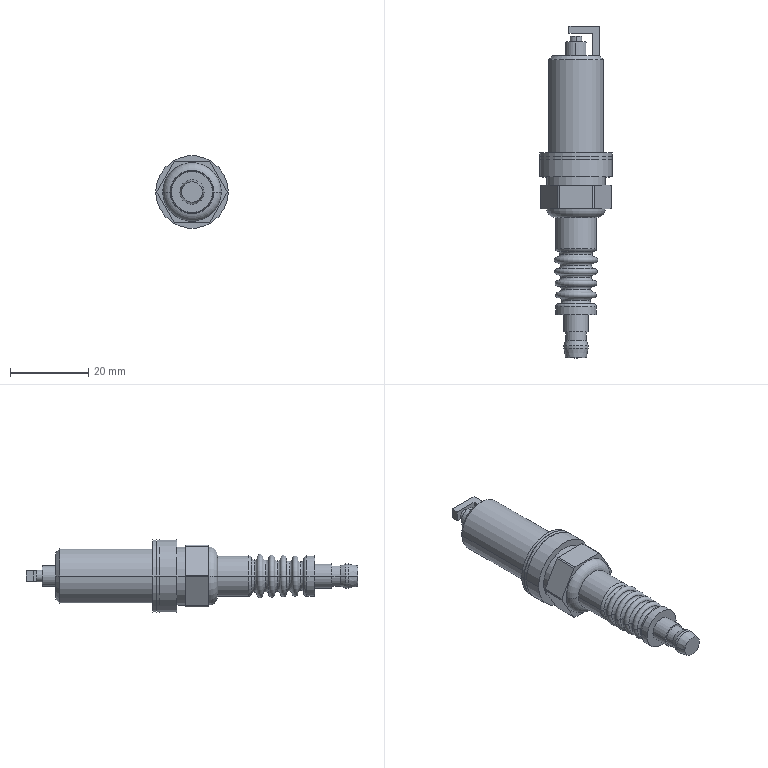Part | STEP file | FR8SES | 3 solids | 104 faces | box 18.6 x 85.1 x 18.6 mm | volume 9845 mm3 | cylinder 35 | torus 34 | plane 29 | cone 6 | commonest cylinder face diameters 18 x7 18.6 x6 6.2 x4 10.5 x4 14.1 x4 3 x2